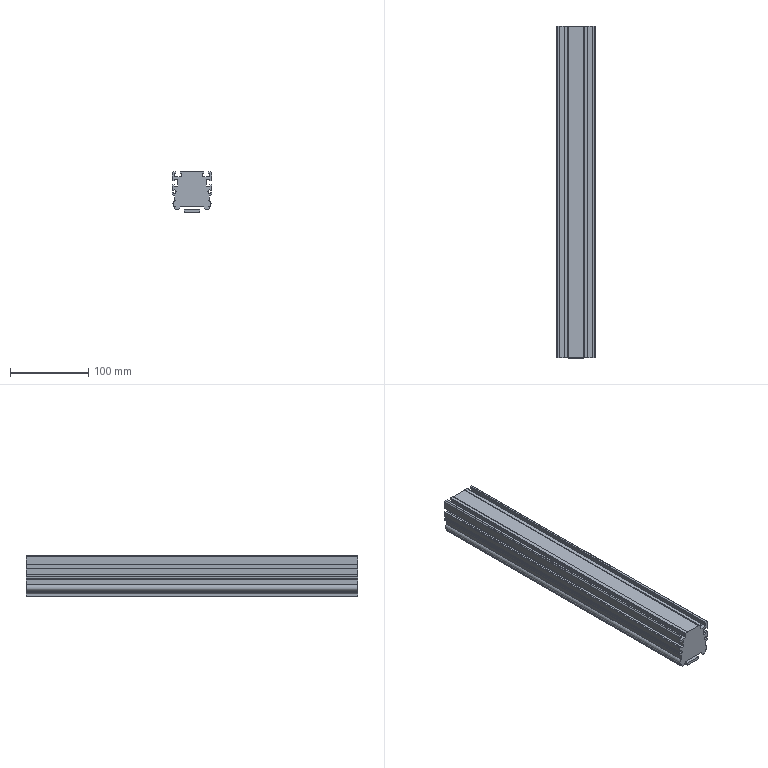Part | STEP file | Copy of 50-2016 profile^K50A-1H20-S(formula driven)-L300-motor left- | 2 solids | 143 faces | box 50 x 425 x 52.45 mm | volume 861534 mm3 | plane 72 | cylinder 71 | commonest cylinder face diameters 0.4 x58 4.2 x6 4 x5 8 x2